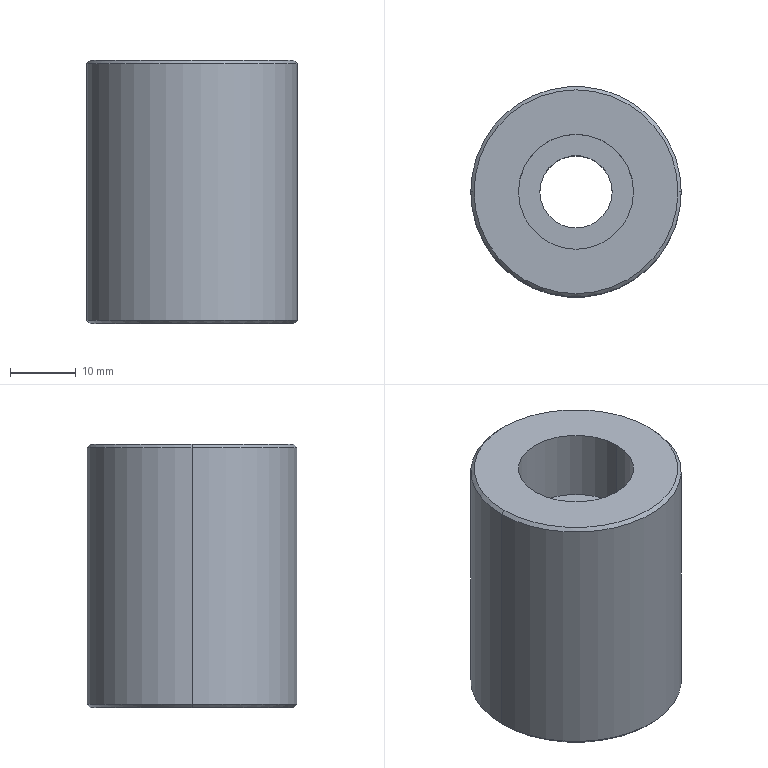Part | Creo | 1 solid | 13 faces | box 32 x 32 x 40 mm | volume 26743 mm3 | cylinder 6 | cone 4 | plane 3 | commonest cylinder face diameters 11 x2 17.5 x2 32 x2
STEP:
#1=CARTESIAN_POINT('',(0.,0.,0.));
#2=DIRECTION('',(0.,0.,1.));
#3=DIRECTION('',(1.,0.,0.));
#4=AXIS2_PLACEMENT_3D('',#1,#2,#3);
#5=CARTESIAN_POINT('',(40.5,-153.,-160.5));
#6=VERTEX_POINT('',#5);
#7=CARTESIAN_POINT('',(71.5,-153.,-160.5));
#8=VERTEX_POINT('',#7);
#9=CARTESIAN_POINT('',(56.,-153.,-160.5));
#10=DIRECTION('',(0.,0.,1.));
#11=DIRECTION('',(-1.,0.,0.));
#12=AXIS2_PLACEMENT_3D('',#9,#10,#11);
#13=CIRCLE('',#12,15.5);
#14=EDGE_CURVE('',#6,#8,#13,.T.);
#15=ORIENTED_EDGE('',*,*,#14,.F.);
#16=CARTESIAN_POINT('',(56.,-153.,-160.5));
#17=DIRECTION('',(0.,0.,1.));
#18=DIRECTION('',(1.,0.,0.));
#19=AXIS2_PLACEMENT_3D('',#16,#17,#18);
#20=CIRCLE('',#19,15.5);
#21=EDGE_CURVE('',#8,#6,#20,.T.);
#22=ORIENTED_EDGE('',*,*,#21,.F.);
#23=EDGE_LOOP('',(#15,#22));
#24=FACE_OUTER_BOUND('',#23,.F.);
#25=CARTESIAN_POINT('',(64.75,-153.,-160.5));
#26=VERTEX_POINT('',#25);
#27=CARTESIAN_POINT('',(47.25,-153.,-160.5));
#28=VERTEX_POINT('',#27);
#29=CARTESIAN_POINT('',(56.,-153.,-160.5));
#30=DIRECTION('',(0.,0.,-1.));
#31=DIRECTION('',(1.,0.,0.));
#32=AXIS2_PLACEMENT_3D('',#29,#30,#31);
#33=CIRCLE('',#32,8.75);
#34=EDGE_CURVE('',#26,#28,#33,.T.);
#35=ORIENTED_EDGE('',*,*,#34,.F.);
#36=CARTESIAN_POINT('',(56.,-153.,-160.5));
#37=DIRECTION('',(0.,0.,-1.));
#38=DIRECTION('',(-1.,0.,0.));
#39=AXIS2_PLACEMENT_3D('',#36,#37,#38);
#40=CIRCLE('',#39,8.75);
#41=EDGE_CURVE('',#28,#26,#40,.T.);
#42=ORIENTED_EDGE('',*,*,#41,.F.);
#43=EDGE_LOOP('',(#35,#42));
#44=FACE_BOUND('',#43,.F.);
#45=CARTESIAN_POINT('',(56.,-153.,-160.5));
#46=DIRECTION('',(0.,0.,-1.));
#47=DIRECTION('',(-1.,0.,0.));
#48=AXIS2_PLACEMENT_3D('',#45,#46,#47);
#49=PLANE('',#48);
#50=ADVANCED_FACE('',(#24,#44),#49,.F.);
#51=ORIENTED_EDGE('',*,*,#14,.T.);
#52=CARTESIAN_POINT('',(72.,-153.,-161.));
#53=VERTEX_POINT('',#52);
#54=CARTESIAN_POINT('',(71.5,-153.,-160.5));
#55=DIRECTION('',(0.7071,0.,-0.7071));
#56=VECTOR('',#55,0.7071);
#57=LINE('',#54,#56);
#58=EDGE_CURVE('',#8,#53,#57,.T.);
#59=ORIENTED_EDGE('',*,*,#58,.T.);
#60=CARTESIAN_POINT('',(40.,-153.,-161.));
#61=VERTEX_POINT('',#60);
#62=CARTESIAN_POINT('',(56.,-153.,-161.));
#63=DIRECTION('',(0.,0.,1.));
#64=DIRECTION('',(-1.,0.,0.));
#65=AXIS2_PLACEMENT_3D('',#62,#63,#64);
#66=CIRCLE('',#65,16.);
#67=EDGE_CURVE('',#61,#53,#66,.T.);
#68=ORIENTED_EDGE('',*,*,#67,.F.);
#69=CARTESIAN_POINT('',(40.5,-153.,-160.5));
#70=DIRECTION('',(-0.7071,0.,-0.7071));
#71=VECTOR('',#70,0.7071);
#72=LINE('',#69,#71);
#73=EDGE_CURVE('',#6,#61,#72,.T.);
#74=ORIENTED_EDGE('',*,*,#73,.F.);
#75=EDGE_LOOP('',(#51,#59,#68,#74));
#76=FACE_OUTER_BOUND('',#75,.F.);
#77=CARTESIAN_POINT('',(56.,-153.,-160.75));
#78=DIRECTION('',(0.,0.,-1.));
#79=DIRECTION('',(-1.,0.,0.));
#80=AXIS2_PLACEMENT_3D('',#77,#78,#79);
#81=CONICAL_SURFACE('',#80,15.75,45.);
#82=ADVANCED_FACE('',(#76),#81,.T.);
#83=ORIENTED_EDGE('',*,*,#21,.T.);
#84=ORIENTED_EDGE('',*,*,#73,.T.);
#85=CARTESIAN_POINT('',(56.,-153.,-161.));
#86=DIRECTION('',(0.,0.,1.));
#87=DIRECTION('',(1.,0.,0.));
#88=AXIS2_PLACEMENT_3D('',#85,#86,#87);
#89=CIRCLE('',#88,16.);
#90=EDGE_CURVE('',#53,#61,#89,.T.);
#91=ORIENTED_EDGE('',*,*,#90,.F.);
#92=ORIENTED_EDGE('',*,*,#58,.F.);
#93=EDGE_LOOP('',(#83,#84,#91,#92));
#94=FACE_OUTER_BOUND('',#93,.F.);
#95=CARTESIAN_POINT('',(56.,-153.,-160.75));
#96=DIRECTION('',(0.,0.,-1.));
#97=DIRECTION('',(-1.,0.,0.));
#98=AXIS2_PLACEMENT_3D('',#95,#96,#97);
#99=CONICAL_SURFACE('',#98,15.75,45.);
#100=ADVANCED_FACE('',(#94),#99,.T.);
#101=CARTESIAN_POINT('',(40.,-153.,-200.));
#102=VERTEX_POINT('',#101);
#103=CARTESIAN_POINT('',(72.,-153.,-200.));
#104=VERTEX_POINT('',#103);
#105=CARTESIAN_POINT('',(56.,-153.,-200.));
#106=DIRECTION('',(0.,0.,-1.));
#107=DIRECTION('',(-1.,0.,0.));
#108=AXIS2_PLACEMENT_3D('',#105,#106,#107);
#109=CIRCLE('',#108,16.);
#110=EDGE_CURVE('',#102,#104,#109,.T.);
#111=ORIENTED_EDGE('',*,*,#110,.T.);
#112=CARTESIAN_POINT('',(72.,-153.,-161.));
#113=DIRECTION('',(0.,0.,-1.));
#114=VECTOR('',#113,39.);
#115=LINE('',#112,#114);
#116=EDGE_CURVE('',#53,#104,#115,.T.);
#117=ORIENTED_EDGE('',*,*,#116,.F.);
#118=ORIENTED_EDGE('',*,*,#90,.T.);
#119=CARTESIAN_POINT('',(40.,-153.,-161.));
#120=DIRECTION('',(0.,0.,-1.));
#121=VECTOR('',#120,39.);
#122=LINE('',#119,#121);
#123=EDGE_CURVE('',#61,#102,#122,.T.);
#124=ORIENTED_EDGE('',*,*,#123,.T.);
#125=EDGE_LOOP('',(#111,#117,#118,#124));
#126=FACE_OUTER_BOUND('',#125,.F.);
#127=CARTESIAN_POINT('',(56.,-153.,-160.5));
#128=DIRECTION('',(0.,0.,-1.));
#129=DIRECTION('',(-1.,0.,0.));
#130=AXIS2_PLACEMENT_3D('',#127,#128,#129);
#131=CYLINDRICAL_SURFACE('',#130,16.);
#132=ADVANCED_FACE('',(#126),#131,.T.);
#133=ORIENTED_EDGE('',*,*,#110,.F.);
#134=CARTESIAN_POINT('',(40.5,-153.,-200.5));
#135=VERTEX_POINT('',#134);
#136=CARTESIAN_POINT('',(40.5,-153.,-200.5));
#137=DIRECTION('',(-0.7071,0.,0.7071));
#138=VECTOR('',#137,0.7071);
#139=LINE('',#136,#138);
#140=EDGE_CURVE('',#135,#102,#139,.T.);
#141=ORIENTED_EDGE('',*,*,#140,.F.);
#142=CARTESIAN_POINT('',(71.5,-153.,-200.5));
#143=VERTEX_POINT('',#142);
#144=CARTESIAN_POINT('',(56.,-153.,-200.5));
#145=DIRECTION('',(0.,0.,-1.));
#146=DIRECTION('',(-1.,0.,0.));
#147=AXIS2_PLACEMENT_3D('',#144,#145,#146);
#148=CIRCLE('',#147,15.5);
#149=EDGE_CURVE('',#135,#143,#148,.T.);
#150=ORIENTED_EDGE('',*,*,#149,.T.);
#151=CARTESIAN_POINT('',(71.5,-153.,-200.5));
#152=DIRECTION('',(0.7071,0.,0.7071));
#153=VECTOR('',#152,0.7071);
#154=LINE('',#151,#153);
#155=EDGE_CURVE('',#143,#104,#154,.T.);
#156=ORIENTED_EDGE('',*,*,#155,.T.);
#157=EDGE_LOOP('',(#133,#141,#150,#156));
#158=FACE_OUTER_BOUND('',#157,.F.);
#159=CARTESIAN_POINT('',(56.,-153.,-200.25));
#160=DIRECTION('',(0.,0.,1.));
#161=DIRECTION('',(1.,0.,0.));
#162=AXIS2_PLACEMENT_3D('',#159,#160,#161);
#163=CONICAL_SURFACE('',#162,15.75,45.);
#164=ADVANCED_FACE('',(#158),#163,.T.);
#165=CARTESIAN_POINT('',(56.,-153.,-200.));
#166=DIRECTION('',(0.,0.,-1.));
#167=DIRECTION('',(1.,0.,0.));
#168=AXIS2_PLACEMENT_3D('',#165,#166,#167);
#169=CIRCLE('',#168,16.);
#170=EDGE_CURVE('',#104,#102,#169,.T.);
#171=ORIENTED_EDGE('',*,*,#170,.F.);
#172=ORIENTED_EDGE('',*,*,#155,.F.);
#173=CARTESIAN_POINT('',(56.,-153.,-200.5));
#174=DIRECTION('',(0.,0.,-1.));
#175=DIRECTION('',(1.,0.,0.));
#176=AXIS2_PLACEMENT_3D('',#173,#174,#175);
#177=CIRCLE('',#176,15.5);
#178=EDGE_CURVE('',#143,#135,#177,.T.);
#179=ORIENTED_EDGE('',*,*,#178,.T.);
#180=ORIENTED_EDGE('',*,*,#140,.T.);
#181=EDGE_LOOP('',(#171,#172,#179,#180));
#182=FACE_OUTER_BOUND('',#181,.F.);
#183=CARTESIAN_POINT('',(56.,-153.,-200.25));
#184=DIRECTION('',(0.,0.,1.));
#185=DIRECTION('',(1.,0.,0.));
#186=AXIS2_PLACEMENT_3D('',#183,#184,#185);
#187=CONICAL_SURFACE('',#186,15.75,45.);
#188=ADVANCED_FACE('',(#182),#187,.T.);
#189=ORIENTED_EDGE('',*,*,#170,.T.);
#190=ORIENTED_EDGE('',*,*,#123,.F.);
#191=ORIENTED_EDGE('',*,*,#67,.T.);
#192=ORIENTED_EDGE('',*,*,#116,.T.);
#193=EDGE_LOOP('',(#189,#190,#191,#192));
#194=FACE_OUTER_BOUND('',#193,.F.);
#195=CARTESIAN_POINT('',(56.,-153.,-160.5));
#196=DIRECTION('',(0.,0.,-1.));
#197=DIRECTION('',(-1.,0.,0.));
#198=AXIS2_PLACEMENT_3D('',#195,#196,#197);
#199=CYLINDRICAL_SURFACE('',#198,16.);
#200=ADVANCED_FACE('',(#194),#199,.T.);
#201=ORIENTED_EDGE('',*,*,#149,.F.);
#202=ORIENTED_EDGE('',*,*,#178,.F.);
#203=EDGE_LOOP('',(#201,#202));
#204=FACE_OUTER_BOUND('',#203,.F.);
#205=CARTESIAN_POINT('',(61.5,-153.,-200.5));
#206=VERTEX_POINT('',#205);
#207=CARTESIAN_POINT('',(50.5,-153.,-200.5));
#208=VERTEX_POINT('',#207);
#209=CARTESIAN_POINT('',(56.,-153.,-200.5));
#210=DIRECTION('',(0.,0.,1.));
#211=DIRECTION('',(1.,0.,0.));
#212=AXIS2_PLACEMENT_3D('',#209,#210,#211);
#213=CIRCLE('',#212,5.5);
#214=EDGE_CURVE('',#206,#208,#213,.T.);
#215=ORIENTED_EDGE('',*,*,#214,.F.);
#216=CARTESIAN_POINT('',(56.,-153.,-200.5));
#217=DIRECTION('',(0.,0.,1.));
#218=DIRECTION('',(-1.,0.,0.));
#219=AXIS2_PLACEMENT_3D('',#216,#217,#218);
#220=CIRCLE('',#219,5.5);
#221=EDGE_CURVE('',#208,#206,#220,.T.);
#222=ORIENTED_EDGE('',*,*,#221,.F.);
#223=EDGE_LOOP('',(#215,#222));
#224=FACE_BOUND('',#223,.F.);
#225=CARTESIAN_POINT('',(56.,-153.,-200.5));
#226=DIRECTION('',(0.,0.,-1.));
#227=DIRECTION('',(-1.,0.,0.));
#228=AXIS2_PLACEMENT_3D('',#225,#226,#227);
#229=PLANE('',#228);
#230=ADVANCED_FACE('',(#204,#224),#229,.T.);
#231=ORIENTED_EDGE('',*,*,#214,.T.);
#232=CARTESIAN_POINT('',(50.5,-153.,-171.5));
#233=VERTEX_POINT('',#232);
#234=CARTESIAN_POINT('',(50.5,-153.,-200.5));
#235=DIRECTION('',(0.,0.,1.));
#236=VECTOR('',#235,29.);
#237=LINE('',#234,#236);
#238=EDGE_CURVE('',#208,#233,#237,.T.);
#239=ORIENTED_EDGE('',*,*,#238,.T.);
#240=CARTESIAN_POINT('',(61.5,-153.,-171.5));
#241=VERTEX_POINT('',#240);
#242=CARTESIAN_POINT('',(56.,-153.,-171.5));
#243=DIRECTION('',(0.,0.,-1.));
#244=DIRECTION('',(-1.,0.,0.));
#245=AXIS2_PLACEMENT_3D('',#242,#243,#244);
#246=CIRCLE('',#245,5.5);
#247=EDGE_CURVE('',#233,#241,#246,.T.);
#248=ORIENTED_EDGE('',*,*,#247,.T.);
#249=CARTESIAN_POINT('',(61.5,-153.,-200.5));
#250=DIRECTION('',(0.,0.,1.));
#251=VECTOR('',#250,29.);
#252=LINE('',#249,#251);
#253=EDGE_CURVE('',#206,#241,#252,.T.);
#254=ORIENTED_EDGE('',*,*,#253,.F.);
#255=EDGE_LOOP('',(#231,#239,#248,#254));
#256=FACE_OUTER_BOUND('',#255,.F.);
#257=CARTESIAN_POINT('',(56.,-153.,-160.5));
#258=DIRECTION('',(0.,0.,1.));
#259=DIRECTION('',(1.,0.,0.));
#260=AXIS2_PLACEMENT_3D('',#257,#258,#259);
#261=CYLINDRICAL_SURFACE('',#260,5.5);
#262=ADVANCED_FACE('',(#256),#261,.F.);
#263=ORIENTED_EDGE('',*,*,#221,.T.);
#264=ORIENTED_EDGE('',*,*,#253,.T.);
#265=CARTESIAN_POINT('',(56.,-153.,-171.5));
#266=DIRECTION('',(0.,0.,-1.));
#267=DIRECTION('',(1.,0.,0.));
#268=AXIS2_PLACEMENT_3D('',#265,#266,#267);
#269=CIRCLE('',#268,5.5);
#270=EDGE_CURVE('',#241,#233,#269,.T.);
#271=ORIENTED_EDGE('',*,*,#270,.T.);
#272=ORIENTED_EDGE('',*,*,#238,.F.);
#273=EDGE_LOOP('',(#263,#264,#271,#272));
#274=FACE_OUTER_BOUND('',#273,.F.);
#275=CARTESIAN_POINT('',(56.,-153.,-160.5));
#276=DIRECTION('',(0.,0.,1.));
#277=DIRECTION('',(1.,0.,0.));
#278=AXIS2_PLACEMENT_3D('',#275,#276,#277);
#279=CYLINDRICAL_SURFACE('',#278,5.5);
#280=ADVANCED_FACE('',(#274),#279,.F.);
#281=CARTESIAN_POINT('',(64.75,-153.,-171.5));
#282=VERTEX_POINT('',#281);
#283=CARTESIAN_POINT('',(47.25,-153.,-171.5));
#284=VERTEX_POINT('',#283);
#285=CARTESIAN_POINT('',(56.,-153.,-171.5));
#286=DIRECTION('',(0.,0.,1.));
#287=DIRECTION('',(1.,0.,0.));
#288=AXIS2_PLACEMENT_3D('',#285,#286,#287);
#289=CIRCLE('',#288,8.75);
#290=EDGE_CURVE('',#282,#284,#289,.T.);
#291=ORIENTED_EDGE('',*,*,#290,.F.);
#292=CARTESIAN_POINT('',(56.,-153.,-171.5));
#293=DIRECTION('',(0.,0.,1.));
#294=DIRECTION('',(-1.,0.,0.));
#295=AXIS2_PLACEMENT_3D('',#292,#293,#294);
#296=CIRCLE('',#295,8.75);
#297=EDGE_CURVE('',#284,#282,#296,.T.);
#298=ORIENTED_EDGE('',*,*,#297,.F.);
#299=EDGE_LOOP('',(#291,#298));
#300=FACE_OUTER_BOUND('',#299,.F.);
#301=ORIENTED_EDGE('',*,*,#270,.F.);
#302=ORIENTED_EDGE('',*,*,#247,.F.);
#303=EDGE_LOOP('',(#301,#302));
#304=FACE_BOUND('',#303,.F.);
#305=CARTESIAN_POINT('',(56.,-144.25,-171.5));
#306=DIRECTION('',(0.,0.,-1.));
#307=DIRECTION('',(-1.,0.,0.));
#308=AXIS2_PLACEMENT_3D('',#305,#306,#307);
#309=PLANE('',#308);
#310=ADVANCED_FACE('',(#300,#304),#309,.F.);
#311=ORIENTED_EDGE('',*,*,#290,.T.);
#312=CARTESIAN_POINT('',(47.25,-153.,-171.5));
#313=DIRECTION('',(0.,0.,1.));
#314=VECTOR('',#313,11.);
#315=LINE('',#312,#314);
#316=EDGE_CURVE('',#284,#28,#315,.T.);
#317=ORIENTED_EDGE('',*,*,#316,.T.);
#318=ORIENTED_EDGE('',*,*,#41,.T.);
#319=CARTESIAN_POINT('',(64.75,-153.,-171.5));
#320=DIRECTION('',(0.,0.,1.));
#321=VECTOR('',#320,11.);
#322=LINE('',#319,#321);
#323=EDGE_CURVE('',#282,#26,#322,.T.);
#324=ORIENTED_EDGE('',*,*,#323,.F.);
#325=EDGE_LOOP('',(#311,#317,#318,#324));
#326=FACE_OUTER_BOUND('',#325,.F.);
#327=CARTESIAN_POINT('',(56.,-153.,-160.5));
#328=DIRECTION('',(0.,0.,1.));
#329=DIRECTION('',(1.,0.,0.));
#330=AXIS2_PLACEMENT_3D('',#327,#328,#329);
#331=CYLINDRICAL_SURFACE('',#330,8.75);
#332=ADVANCED_FACE('',(#326),#331,.F.);
#333=ORIENTED_EDGE('',*,*,#297,.T.);
#334=ORIENTED_EDGE('',*,*,#323,.T.);
#335=ORIENTED_EDGE('',*,*,#34,.T.);
#336=ORIENTED_EDGE('',*,*,#316,.F.);
#337=EDGE_LOOP('',(#333,#334,#335,#336));
#338=FACE_OUTER_BOUND('',#337,.F.);
#339=CARTESIAN_POINT('',(56.,-153.,-160.5));
#340=DIRECTION('',(0.,0.,1.));
#341=DIRECTION('',(1.,0.,0.));
#342=AXIS2_PLACEMENT_3D('',#339,#340,#341);
#343=CYLINDRICAL_SURFACE('',#342,8.75);
#344=ADVANCED_FACE('',(#338),#343,.F.);
#345=CLOSED_SHELL('',(#50,#82,#100,#132,#164,#188,#200,#230,#262,#280,#310,#332,#344));
#346=MANIFOLD_SOLID_BREP('',#345);
#347=(LENGTH_UNIT()NAMED_UNIT(*)SI_UNIT(.MILLI.,.METRE.));
#348=UNCERTAINTY_MEASURE_WITH_UNIT(LENGTH_MEASURE(0.00604),#347,'','');
#349=(NAMED_UNIT(*)PLANE_ANGLE_UNIT()SI_UNIT($,.RADIAN.));
#350=PLANE_ANGLE_MEASURE_WITH_UNIT(PLANE_ANGLE_MEASURE(0.01745),#349);
#351=(CONVERSION_BASED_UNIT('DEGREE',#350)NAMED_UNIT(*)PLANE_ANGLE_UNIT());
#352=(NAMED_UNIT(*)SI_UNIT($,.STERADIAN.)SOLID_ANGLE_UNIT());
#353=(GEOMETRIC_REPRESENTATION_CONTEXT(3)GLOBAL_UNCERTAINTY_ASSIGNED_CONTEXT((#348))GLOBAL_UNIT_ASSIGNED_CONTEXT((#347,#351,#352))REPRESENTATION_CONTEXT('',''));
#354=ADVANCED_BREP_SHAPE_REPRESENTATION('',(#4,#346),#353);